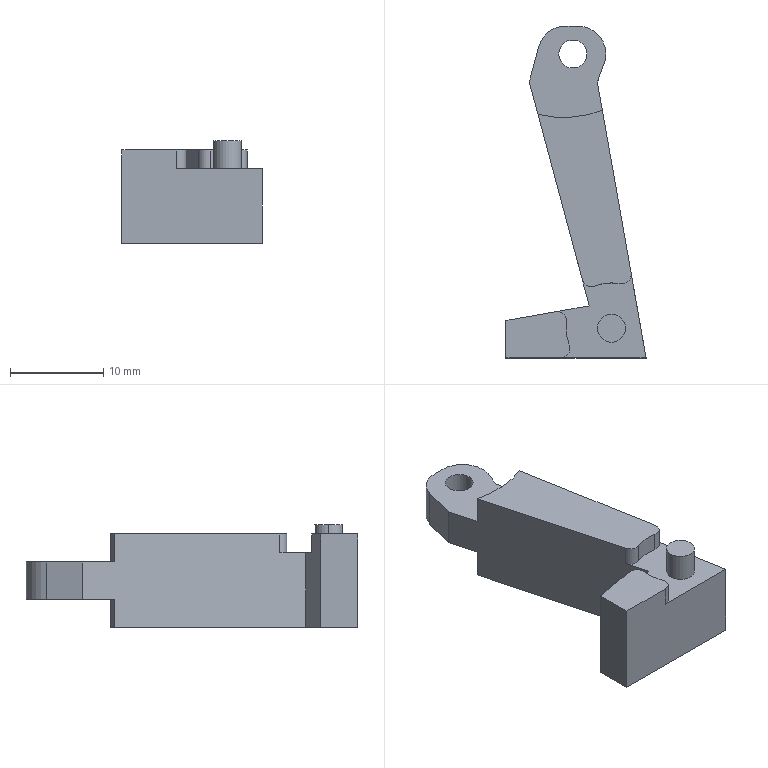Part | SolidWorks | features ICE 14, Fillet 5, MirrorPattern 2, Extrusion 1 | 1 solid | 33 faces | box 15 x 35.544 x 11 mm | volume 2110 mm3 | cylinder 18 | plane 15 | commonest cylinder face diameters 2 x7 3 x4 6 x3 9.731 x2 23.6 x2
STEP:
#1=CARTESIAN_POINT('',(13.411,8.923,8.));
#2=VERTEX_POINT('',#1);
#3=CARTESIAN_POINT('',(12.222,7.941,8.));
#4=VERTEX_POINT('',#3);
#5=CARTESIAN_POINT('',(12.411,8.923,8.));
#6=DIRECTION('',(0.,0.,-1.));
#7=DIRECTION('',(1.,0.,0.));
#8=AXIS2_PLACEMENT_3D('',#5,#6,#7);
#9=CIRCLE('',#8,1.);
#10=EDGE_CURVE('',#2,#4,#9,.T.);
#11=ORIENTED_EDGE('',*,*,#10,.F.);
#12=CARTESIAN_POINT('',(13.411,8.923,10.));
#13=VERTEX_POINT('',#12);
#14=CARTESIAN_POINT('',(13.411,8.923,8.));
#15=DIRECTION('',(0.,0.,1.));
#16=VECTOR('',#15,1000.);
#17=LINE('',#14,#16);
#18=EDGE_CURVE('',#2,#13,#17,.T.);
#19=ORIENTED_EDGE('',*,*,#18,.T.);
#20=CARTESIAN_POINT('',(12.222,7.941,10.));
#21=VERTEX_POINT('',#20);
#22=CARTESIAN_POINT('',(12.411,8.923,10.));
#23=DIRECTION('',(0.,0.,1.));
#24=DIRECTION('',(1.,0.,0.));
#25=AXIS2_PLACEMENT_3D('',#22,#23,#24);
#26=CIRCLE('',#25,1.);
#27=EDGE_CURVE('',#21,#13,#26,.T.);
#28=ORIENTED_EDGE('',*,*,#27,.F.);
#29=CARTESIAN_POINT('',(12.222,7.941,8.));
#30=DIRECTION('',(0.,0.,1.));
#31=VECTOR('',#30,1000.);
#32=LINE('',#29,#31);
#33=EDGE_CURVE('',#4,#21,#32,.T.);
#34=ORIENTED_EDGE('',*,*,#33,.F.);
#35=EDGE_LOOP('',(#11,#19,#28,#34));
#36=FACE_OUTER_BOUND('',#35,.T.);
#37=CARTESIAN_POINT('',(12.411,8.923,8.));
#38=DIRECTION('',(0.,0.,1.));
#39=DIRECTION('',(1.,0.,0.));
#40=AXIS2_PLACEMENT_3D('',#37,#38,#39);
#41=CYLINDRICAL_SURFACE('',#40,1.);
#42=ADVANCED_FACE('',(#36),#41,.T.);
#43=CARTESIAN_POINT('',(6.491,3.953,8.));
#44=VERTEX_POINT('',#43);
#45=CARTESIAN_POINT('',(6.482,3.818,8.));
#46=VERTEX_POINT('',#45);
#47=CARTESIAN_POINT('',(5.491,3.953,8.));
#48=DIRECTION('',(0.,0.,-1.));
#49=DIRECTION('',(1.,0.,0.));
#50=AXIS2_PLACEMENT_3D('',#47,#48,#49);
#51=CIRCLE('',#50,1.);
#52=EDGE_CURVE('',#44,#46,#51,.T.);
#53=ORIENTED_EDGE('',*,*,#52,.F.);
#54=CARTESIAN_POINT('',(6.491,3.953,10.));
#55=VERTEX_POINT('',#54);
#56=CARTESIAN_POINT('',(6.491,3.953,8.));
#57=DIRECTION('',(0.,0.,1.));
#58=VECTOR('',#57,1000.);
#59=LINE('',#56,#58);
#60=EDGE_CURVE('',#44,#55,#59,.T.);
#61=ORIENTED_EDGE('',*,*,#60,.T.);
#62=CARTESIAN_POINT('',(6.482,3.818,10.));
#63=VERTEX_POINT('',#62);
#64=CARTESIAN_POINT('',(5.491,3.953,10.));
#65=DIRECTION('',(0.,0.,1.));
#66=DIRECTION('',(1.,0.,0.));
#67=AXIS2_PLACEMENT_3D('',#64,#65,#66);
#68=CIRCLE('',#67,1.);
#69=EDGE_CURVE('',#63,#55,#68,.T.);
#70=ORIENTED_EDGE('',*,*,#69,.F.);
#71=CARTESIAN_POINT('',(6.482,3.818,8.));
#72=DIRECTION('',(0.,0.,1.));
#73=VECTOR('',#72,1000.);
#74=LINE('',#71,#73);
#75=EDGE_CURVE('',#46,#63,#74,.T.);
#76=ORIENTED_EDGE('',*,*,#75,.F.);
#77=EDGE_LOOP('',(#53,#61,#70,#76));
#78=FACE_OUTER_BOUND('',#77,.T.);
#79=CARTESIAN_POINT('',(5.491,3.953,8.));
#80=DIRECTION('',(0.,0.,1.));
#81=DIRECTION('',(1.,0.,0.));
#82=AXIS2_PLACEMENT_3D('',#79,#80,#81);
#83=CYLINDRICAL_SURFACE('',#82,1.);
#84=ADVANCED_FACE('',(#78),#83,.T.);
#85=CARTESIAN_POINT('',(6.851,1.,8.));
#86=VERTEX_POINT('',#85);
#87=CARTESIAN_POINT('',(5.851,0.,8.));
#88=VERTEX_POINT('',#87);
#89=CARTESIAN_POINT('',(5.851,1.,8.));
#90=DIRECTION('',(0.,0.,-1.));
#91=DIRECTION('',(1.,0.,0.));
#92=AXIS2_PLACEMENT_3D('',#89,#90,#91);
#93=CIRCLE('',#92,1.);
#94=EDGE_CURVE('',#86,#88,#93,.T.);
#95=ORIENTED_EDGE('',*,*,#94,.F.);
#96=CARTESIAN_POINT('',(6.851,1.,10.));
#97=VERTEX_POINT('',#96);
#98=CARTESIAN_POINT('',(6.851,1.,8.));
#99=DIRECTION('',(0.,0.,1.));
#100=VECTOR('',#99,1000.);
#101=LINE('',#98,#100);
#102=EDGE_CURVE('',#86,#97,#101,.T.);
#103=ORIENTED_EDGE('',*,*,#102,.T.);
#104=CARTESIAN_POINT('',(5.851,0.,10.));
#105=VERTEX_POINT('',#104);
#106=CARTESIAN_POINT('',(5.851,1.,10.));
#107=DIRECTION('',(0.,0.,1.));
#108=DIRECTION('',(1.,0.,0.));
#109=AXIS2_PLACEMENT_3D('',#106,#107,#108);
#110=CIRCLE('',#109,1.);
#111=EDGE_CURVE('',#105,#97,#110,.T.);
#112=ORIENTED_EDGE('',*,*,#111,.F.);
#113=CARTESIAN_POINT('',(5.851,0.,10.));
#114=DIRECTION('',(0.,0.,1.));
#115=VECTOR('',#114,1000.);
#116=LINE('',#113,#115);
#117=EDGE_CURVE('',#88,#105,#116,.T.);
#118=ORIENTED_EDGE('',*,*,#117,.F.);
#119=EDGE_LOOP('',(#95,#103,#112,#118));
#120=FACE_OUTER_BOUND('',#119,.T.);
#121=CARTESIAN_POINT('',(5.851,1.,8.));
#122=DIRECTION('',(0.,0.,1.));
#123=DIRECTION('',(1.,0.,0.));
#124=AXIS2_PLACEMENT_3D('',#121,#122,#123);
#125=CYLINDRICAL_SURFACE('',#124,1.);
#126=ADVANCED_FACE('',(#120),#125,.T.);
#127=CARTESIAN_POINT('',(12.803,3.163,11.));
#128=VERTEX_POINT('',#127);
#129=CARTESIAN_POINT('',(9.803,3.163,11.));
#130=VERTEX_POINT('',#129);
#131=CARTESIAN_POINT('',(11.303,3.163,11.));
#132=DIRECTION('',(0.,0.,1.));
#133=DIRECTION('',(1.,0.,0.));
#134=AXIS2_PLACEMENT_3D('',#131,#132,#133);
#135=CIRCLE('',#134,1.5);
#136=EDGE_CURVE('',#128,#130,#135,.T.);
#137=ORIENTED_EDGE('',*,*,#136,.F.);
#138=CARTESIAN_POINT('',(12.803,3.163,8.));
#139=VERTEX_POINT('',#138);
#140=CARTESIAN_POINT('',(12.803,3.163,11.));
#141=DIRECTION('',(0.,0.,-1.));
#142=VECTOR('',#141,1000.);
#143=LINE('',#140,#142);
#144=EDGE_CURVE('',#128,#139,#143,.T.);
#145=ORIENTED_EDGE('',*,*,#144,.T.);
#146=CARTESIAN_POINT('',(9.803,3.163,8.));
#147=VERTEX_POINT('',#146);
#148=CARTESIAN_POINT('',(11.303,3.163,8.));
#149=DIRECTION('',(0.,0.,1.));
#150=DIRECTION('',(1.,0.,0.));
#151=AXIS2_PLACEMENT_3D('',#148,#149,#150);
#152=CIRCLE('',#151,1.5);
#153=EDGE_CURVE('',#139,#147,#152,.T.);
#154=ORIENTED_EDGE('',*,*,#153,.T.);
#155=CARTESIAN_POINT('',(9.803,3.163,11.));
#156=DIRECTION('',(0.,0.,-1.));
#157=VECTOR('',#156,1000.);
#158=LINE('',#155,#157);
#159=EDGE_CURVE('',#130,#147,#158,.T.);
#160=ORIENTED_EDGE('',*,*,#159,.F.);
#161=EDGE_LOOP('',(#137,#145,#154,#160));
#162=FACE_OUTER_BOUND('',#161,.T.);
#163=CARTESIAN_POINT('',(11.303,3.163,11.));
#164=DIRECTION('',(0.,0.,-1.));
#165=DIRECTION('',(-1.,0.,0.));
#166=AXIS2_PLACEMENT_3D('',#163,#164,#165);
#167=CYLINDRICAL_SURFACE('',#166,1.5);
#168=ADVANCED_FACE('',(#162),#167,.T.);
#169=CARTESIAN_POINT('',(8.658,32.544,7.));
#170=VERTEX_POINT('',#169);
#171=CARTESIAN_POINT('',(5.658,32.544,7.));
#172=VERTEX_POINT('',#171);
#173=CARTESIAN_POINT('',(7.158,32.544,7.));
#174=DIRECTION('',(0.,0.,-1.));
#175=DIRECTION('',(0.,-1.,0.));
#176=AXIS2_PLACEMENT_3D('',#173,#174,#175);
#177=CIRCLE('',#176,1.5);
#178=EDGE_CURVE('',#170,#172,#177,.T.);
#179=ORIENTED_EDGE('',*,*,#178,.F.);
#180=CARTESIAN_POINT('',(8.658,32.544,3.));
#181=VERTEX_POINT('',#180);
#182=CARTESIAN_POINT('',(8.658,32.544,30.));
#183=DIRECTION('',(0.,0.,-1.));
#184=VECTOR('',#183,1000.);
#185=LINE('',#182,#184);
#186=EDGE_CURVE('',#170,#181,#185,.T.);
#187=ORIENTED_EDGE('',*,*,#186,.T.);
#188=CARTESIAN_POINT('',(5.658,32.544,3.));
#189=VERTEX_POINT('',#188);
#190=CARTESIAN_POINT('',(7.158,32.544,3.));
#191=DIRECTION('',(0.,0.,1.));
#192=DIRECTION('',(0.,1.,0.));
#193=AXIS2_PLACEMENT_3D('',#190,#191,#192);
#194=CIRCLE('',#193,1.5);
#195=EDGE_CURVE('',#189,#181,#194,.T.);
#196=ORIENTED_EDGE('',*,*,#195,.F.);
#197=CARTESIAN_POINT('',(5.658,32.544,30.));
#198=DIRECTION('',(0.,0.,-1.));
#199=VECTOR('',#198,1000.);
#200=LINE('',#197,#199);
#201=EDGE_CURVE('',#172,#189,#200,.T.);
#202=ORIENTED_EDGE('',*,*,#201,.F.);
#203=EDGE_LOOP('',(#179,#187,#196,#202));
#204=FACE_OUTER_BOUND('',#203,.T.);
#205=CARTESIAN_POINT('',(7.158,32.544,30.));
#206=DIRECTION('',(0.,0.,-1.));
#207=DIRECTION('',(-1.,0.,0.));
#208=AXIS2_PLACEMENT_3D('',#205,#206,#207);
#209=CYLINDRICAL_SURFACE('',#208,1.5);
#210=ADVANCED_FACE('',(#204),#209,.F.);
#211=CARTESIAN_POINT('',(10.509,31.518,3.));
#212=VERTEX_POINT('',#211);
#213=CARTESIAN_POINT('',(10.69,32.544,3.));
#214=VERTEX_POINT('',#213);
#215=CARTESIAN_POINT('',(7.69,32.544,3.));
#216=DIRECTION('',(0.,0.,1.));
#217=DIRECTION('',(0.,1.,0.));
#218=AXIS2_PLACEMENT_3D('',#215,#216,#217);
#219=CIRCLE('',#218,3.);
#220=EDGE_CURVE('',#212,#214,#219,.T.);
#221=ORIENTED_EDGE('',*,*,#220,.T.);
#222=CARTESIAN_POINT('',(10.69,32.544,7.));
#223=VERTEX_POINT('',#222);
#224=CARTESIAN_POINT('',(10.69,32.544,10.));
#225=DIRECTION('',(0.,0.,1.));
#226=VECTOR('',#225,1000.);
#227=LINE('',#224,#226);
#228=EDGE_CURVE('',#214,#223,#227,.T.);
#229=ORIENTED_EDGE('',*,*,#228,.T.);
#230=CARTESIAN_POINT('',(10.509,31.518,7.));
#231=VERTEX_POINT('',#230);
#232=CARTESIAN_POINT('',(7.69,32.544,7.));
#233=DIRECTION('',(0.,0.,-1.));
#234=DIRECTION('',(0.,-1.,0.));
#235=AXIS2_PLACEMENT_3D('',#232,#233,#234);
#236=CIRCLE('',#235,3.);
#237=EDGE_CURVE('',#223,#231,#236,.T.);
#238=ORIENTED_EDGE('',*,*,#237,.T.);
#239=CARTESIAN_POINT('',(10.509,31.518,10.));
#240=DIRECTION('',(0.,0.,1.));
#241=VECTOR('',#240,1000.);
#242=LINE('',#239,#241);
#243=EDGE_CURVE('',#212,#231,#242,.T.);
#244=ORIENTED_EDGE('',*,*,#243,.F.);
#245=EDGE_LOOP('',(#221,#229,#238,#244));
#246=FACE_OUTER_BOUND('',#245,.T.);
#247=CARTESIAN_POINT('',(7.69,32.544,10.));
#248=DIRECTION('',(0.,0.,1.));
#249=DIRECTION('',(1.,0.,0.));
#250=AXIS2_PLACEMENT_3D('',#247,#248,#249);
#251=CYLINDRICAL_SURFACE('',#250,3.);
#252=ADVANCED_FACE('',(#246),#251,.T.);
#253=CARTESIAN_POINT('',(3.431,26.06,10.));
#254=VERTEX_POINT('',#253);
#255=CARTESIAN_POINT('',(8.175,8.356,10.));
#256=VERTEX_POINT('',#255);
#257=CARTESIAN_POINT('',(2.497,29.544,10.));
#258=DIRECTION('',(0.2588,-0.9659,0.));
#259=VECTOR('',#258,1000.);
#260=LINE('',#257,#259);
#261=EDGE_CURVE('',#254,#256,#260,.T.);
#262=ORIENTED_EDGE('',*,*,#261,.T.);
#263=CARTESIAN_POINT('',(9.509,7.686,10.));
#264=VERTEX_POINT('',#263);
#265=CARTESIAN_POINT('',(9.141,8.615,10.));
#266=DIRECTION('',(0.,0.,1.));
#267=DIRECTION('',(1.,0.,0.));
#268=AXIS2_PLACEMENT_3D('',#265,#266,#267);
#269=CIRCLE('',#268,1.);
#270=EDGE_CURVE('',#256,#264,#269,.T.);
#271=ORIENTED_EDGE('',*,*,#270,.T.);
#272=CARTESIAN_POINT('',(11.303,3.163,10.));
#273=DIRECTION('',(0.,0.,1.));
#274=DIRECTION('',(1.,0.,0.));
#275=AXIS2_PLACEMENT_3D('',#272,#273,#274);
#276=CIRCLE('',#275,4.865);
#277=EDGE_CURVE('',#21,#264,#276,.T.);
#278=ORIENTED_EDGE('',*,*,#277,.F.);
#279=ORIENTED_EDGE('',*,*,#27,.T.);
#280=CARTESIAN_POINT('',(13.396,9.097,10.));
#281=VERTEX_POINT('',#280);
#282=CARTESIAN_POINT('',(12.411,8.923,10.));
#283=DIRECTION('',(0.,0.,1.));
#284=DIRECTION('',(1.,0.,0.));
#285=AXIS2_PLACEMENT_3D('',#282,#283,#284);
#286=CIRCLE('',#285,1.);
#287=EDGE_CURVE('',#13,#281,#286,.T.);
#288=ORIENTED_EDGE('',*,*,#287,.T.);
#289=CARTESIAN_POINT('',(10.326,26.51,10.));
#290=VERTEX_POINT('',#289);
#291=CARTESIAN_POINT('',(15.,0.,10.));
#292=DIRECTION('',(-0.1736,0.9848,0.));
#293=VECTOR('',#292,1000.);
#294=LINE('',#291,#293);
#295=EDGE_CURVE('',#281,#290,#294,.T.);
#296=ORIENTED_EDGE('',*,*,#295,.T.);
#297=CARTESIAN_POINT('',(6.144,37.544,10.));
#298=DIRECTION('',(0.,0.,-1.));
#299=DIRECTION('',(-1.,0.,0.));
#300=AXIS2_PLACEMENT_3D('',#297,#298,#299);
#301=CIRCLE('',#300,11.8);
#302=EDGE_CURVE('',#290,#254,#301,.T.);
#303=ORIENTED_EDGE('',*,*,#302,.T.);
#304=EDGE_LOOP('',(#262,#271,#278,#279,#288,#296,#303));
#305=FACE_OUTER_BOUND('',#304,.T.);
#306=CARTESIAN_POINT('',(0.,0.,10.));
#307=DIRECTION('',(0.,0.,1.));
#308=DIRECTION('',(1.,0.,0.));
#309=AXIS2_PLACEMENT_3D('',#306,#307,#308);
#310=PLANE('',#309);
#311=ADVANCED_FACE('',(#305),#310,.T.);
#312=CARTESIAN_POINT('',(0.,0.,10.));
#313=VERTEX_POINT('',#312);
#314=CARTESIAN_POINT('',(0.,0.,10.));
#315=DIRECTION('',(1.,0.,0.));
#316=VECTOR('',#315,1000.);
#317=LINE('',#314,#316);
#318=EDGE_CURVE('',#313,#105,#317,.T.);
#319=ORIENTED_EDGE('',*,*,#318,.T.);
#320=ORIENTED_EDGE('',*,*,#111,.T.);
#321=CARTESIAN_POINT('',(6.781,1.369,10.));
#322=VERTEX_POINT('',#321);
#323=CARTESIAN_POINT('',(5.851,1.,10.));
#324=DIRECTION('',(0.,0.,1.));
#325=DIRECTION('',(1.,0.,0.));
#326=AXIS2_PLACEMENT_3D('',#323,#324,#325);
#327=CIRCLE('',#326,1.);
#328=EDGE_CURVE('',#97,#322,#327,.T.);
#329=ORIENTED_EDGE('',*,*,#328,.T.);
#330=CARTESIAN_POINT('',(11.303,3.163,10.));
#331=DIRECTION('',(0.,0.,1.));
#332=DIRECTION('',(1.,0.,0.));
#333=AXIS2_PLACEMENT_3D('',#330,#331,#332);
#334=CIRCLE('',#333,4.865);
#335=EDGE_CURVE('',#63,#322,#334,.T.);
#336=ORIENTED_EDGE('',*,*,#335,.F.);
#337=ORIENTED_EDGE('',*,*,#69,.T.);
#338=CARTESIAN_POINT('',(5.318,4.938,10.));
#339=VERTEX_POINT('',#338);
#340=CARTESIAN_POINT('',(5.491,3.953,10.));
#341=DIRECTION('',(0.,0.,1.));
#342=DIRECTION('',(1.,0.,0.));
#343=AXIS2_PLACEMENT_3D('',#340,#341,#342);
#344=CIRCLE('',#343,1.);
#345=EDGE_CURVE('',#55,#339,#344,.T.);
#346=ORIENTED_EDGE('',*,*,#345,.T.);
#347=CARTESIAN_POINT('',(0.,4.,10.));
#348=VERTEX_POINT('',#347);
#349=CARTESIAN_POINT('',(8.921,5.573,10.));
#350=DIRECTION('',(-0.9848,-0.1736,0.));
#351=VECTOR('',#350,1000.);
#352=LINE('',#349,#351);
#353=EDGE_CURVE('',#339,#348,#352,.T.);
#354=ORIENTED_EDGE('',*,*,#353,.T.);
#355=CARTESIAN_POINT('',(0.,4.,10.));
#356=DIRECTION('',(0.,-1.,0.));
#357=VECTOR('',#356,1000.);
#358=LINE('',#355,#357);
#359=EDGE_CURVE('',#348,#313,#358,.T.);
#360=ORIENTED_EDGE('',*,*,#359,.T.);
#361=EDGE_LOOP('',(#319,#320,#329,#336,#337,#346,#354,#360));
#362=FACE_OUTER_BOUND('',#361,.T.);
#363=CARTESIAN_POINT('',(0.,0.,10.));
#364=DIRECTION('',(0.,0.,1.));
#365=DIRECTION('',(1.,0.,0.));
#366=AXIS2_PLACEMENT_3D('',#363,#364,#365);
#367=PLANE('',#366);
#368=ADVANCED_FACE('',(#362),#367,.T.);
#369=ORIENTED_EDGE('',*,*,#295,.F.);
#370=CARTESIAN_POINT('',(13.396,9.097,8.));
#371=VERTEX_POINT('',#370);
#372=CARTESIAN_POINT('',(13.396,9.097,10.));
#373=DIRECTION('',(0.,0.,-1.));
#374=VECTOR('',#373,1000.);
#375=LINE('',#372,#374);
#376=EDGE_CURVE('',#281,#371,#375,.T.);
#377=ORIENTED_EDGE('',*,*,#376,.T.);
#378=CARTESIAN_POINT('',(15.,0.,8.));
#379=VERTEX_POINT('',#378);
#380=CARTESIAN_POINT('',(15.,0.,8.));
#381=DIRECTION('',(-0.1736,0.9848,0.));
#382=VECTOR('',#381,1000.);
#383=LINE('',#380,#382);
#384=EDGE_CURVE('',#379,#371,#383,.T.);
#385=ORIENTED_EDGE('',*,*,#384,.F.);
#386=CARTESIAN_POINT('',(15.,0.,0.));
#387=VERTEX_POINT('',#386);
#388=CARTESIAN_POINT('',(15.,0.,10.));
#389=DIRECTION('',(0.,0.,-1.));
#390=VECTOR('',#389,1000.);
#391=LINE('',#388,#390);
#392=EDGE_CURVE('',#379,#387,#391,.T.);
#393=ORIENTED_EDGE('',*,*,#392,.T.);
#394=CARTESIAN_POINT('',(10.326,26.51,0.));
#395=VERTEX_POINT('',#394);
#396=CARTESIAN_POINT('',(15.,0.,0.));
#397=DIRECTION('',(-0.1736,0.9848,0.));
#398=VECTOR('',#397,1000.);
#399=LINE('',#396,#398);
#400=EDGE_CURVE('',#387,#395,#399,.T.);
#401=ORIENTED_EDGE('',*,*,#400,.T.);
#402=CARTESIAN_POINT('',(10.326,26.51,3.));
#403=VERTEX_POINT('',#402);
#404=CARTESIAN_POINT('',(10.326,26.51,3.));
#405=DIRECTION('',(0.,0.,-1.));
#406=VECTOR('',#405,1000.);
#407=LINE('',#404,#406);
#408=EDGE_CURVE('',#403,#395,#407,.T.);
#409=ORIENTED_EDGE('',*,*,#408,.F.);
#410=CARTESIAN_POINT('',(9.791,29.544,3.));
#411=VERTEX_POINT('',#410);
#412=CARTESIAN_POINT('',(14.548,2.565,3.));
#413=DIRECTION('',(0.1736,-0.9848,0.));
#414=VECTOR('',#413,1000.);
#415=LINE('',#412,#414);
#416=EDGE_CURVE('',#411,#403,#415,.T.);
#417=ORIENTED_EDGE('',*,*,#416,.F.);
#418=CARTESIAN_POINT('',(9.791,29.544,7.));
#419=VERTEX_POINT('',#418);
#420=CARTESIAN_POINT('',(9.791,29.544,10.));
#421=DIRECTION('',(0.,0.,-1.));
#422=VECTOR('',#421,1000.);
#423=LINE('',#420,#422);
#424=EDGE_CURVE('',#419,#411,#423,.T.);
#425=ORIENTED_EDGE('',*,*,#424,.F.);
#426=CARTESIAN_POINT('',(10.326,26.51,7.));
#427=VERTEX_POINT('',#426);
#428=CARTESIAN_POINT('',(14.548,2.565,7.));
#429=DIRECTION('',(0.1736,-0.9848,0.));
#430=VECTOR('',#429,1000.);
#431=LINE('',#428,#430);
#432=EDGE_CURVE('',#419,#427,#431,.T.);
#433=ORIENTED_EDGE('',*,*,#432,.T.);
#434=CARTESIAN_POINT('',(10.326,26.51,7.));
#435=DIRECTION('',(0.,0.,1.));
#436=VECTOR('',#435,1000.);
#437=LINE('',#434,#436);
#438=EDGE_CURVE('',#427,#290,#437,.T.);
#439=ORIENTED_EDGE('',*,*,#438,.T.);
#440=EDGE_LOOP('',(#369,#377,#385,#393,#401,#409,#417,#425,#433,#439));
#441=FACE_OUTER_BOUND('',#440,.T.);
#442=CARTESIAN_POINT('',(15.,0.,10.));
#443=DIRECTION('',(-0.9848,-0.1736,0.));
#444=DIRECTION('',(0.1736,-0.9848,0.));
#445=AXIS2_PLACEMENT_3D('',#442,#443,#444);
#446=PLANE('',#445);
#447=ADVANCED_FACE('',(#441),#446,.F.);
#448=CARTESIAN_POINT('',(8.175,8.356,8.));
#449=VERTEX_POINT('',#448);
#450=CARTESIAN_POINT('',(8.921,5.573,8.));
#451=VERTEX_POINT('',#450);
#452=CARTESIAN_POINT('',(2.497,29.544,8.));
#453=DIRECTION('',(0.2588,-0.9659,0.));
#454=VECTOR('',#453,1000.);
#455=LINE('',#452,#454);
#456=EDGE_CURVE('',#449,#451,#455,.T.);
#457=ORIENTED_EDGE('',*,*,#456,.F.);
#458=CARTESIAN_POINT('',(8.175,8.356,10.));
#459=DIRECTION('',(0.,0.,1.));
#460=VECTOR('',#459,1000.);
#461=LINE('',#458,#460);
#462=EDGE_CURVE('',#449,#256,#461,.T.);
#463=ORIENTED_EDGE('',*,*,#462,.T.);
#464=ORIENTED_EDGE('',*,*,#261,.F.);
#465=CARTESIAN_POINT('',(3.431,26.06,7.));
#466=VERTEX_POINT('',#465);
#467=CARTESIAN_POINT('',(3.431,26.06,7.));
#468=DIRECTION('',(0.,0.,1.));
#469=VECTOR('',#468,1000.);
#470=LINE('',#467,#469);
#471=EDGE_CURVE('',#466,#254,#470,.T.);
#472=ORIENTED_EDGE('',*,*,#471,.F.);
#473=CARTESIAN_POINT('',(2.497,29.544,7.));
#474=VERTEX_POINT('',#473);
#475=CARTESIAN_POINT('',(9.716,2.603,7.));
#476=DIRECTION('',(-0.2588,0.9659,0.));
#477=VECTOR('',#476,1000.);
#478=LINE('',#475,#477);
#479=EDGE_CURVE('',#466,#474,#478,.T.);
#480=ORIENTED_EDGE('',*,*,#479,.T.);
#481=CARTESIAN_POINT('',(2.497,29.544,3.));
#482=VERTEX_POINT('',#481);
#483=CARTESIAN_POINT('',(2.497,29.544,10.));
#484=DIRECTION('',(0.,0.,-1.));
#485=VECTOR('',#484,1000.);
#486=LINE('',#483,#485);
#487=EDGE_CURVE('',#474,#482,#486,.T.);
#488=ORIENTED_EDGE('',*,*,#487,.T.);
#489=CARTESIAN_POINT('',(3.431,26.06,3.));
#490=VERTEX_POINT('',#489);
#491=CARTESIAN_POINT('',(9.716,2.603,3.));
#492=DIRECTION('',(-0.2588,0.9659,0.));
#493=VECTOR('',#492,1000.);
#494=LINE('',#491,#493);
#495=EDGE_CURVE('',#490,#482,#494,.T.);
#496=ORIENTED_EDGE('',*,*,#495,.F.);
#497=CARTESIAN_POINT('',(3.431,26.06,0.));
#498=VERTEX_POINT('',#497);
#499=CARTESIAN_POINT('',(3.431,26.06,3.));
#500=DIRECTION('',(0.,0.,-1.));
#501=VECTOR('',#500,1000.);
#502=LINE('',#499,#501);
#503=EDGE_CURVE('',#490,#498,#502,.T.);
#504=ORIENTED_EDGE('',*,*,#503,.T.);
#505=CARTESIAN_POINT('',(8.921,5.573,0.));
#506=VERTEX_POINT('',#505);
#507=CARTESIAN_POINT('',(2.497,29.544,0.));
#508=DIRECTION('',(0.2588,-0.9659,0.));
#509=VECTOR('',#508,1000.);
#510=LINE('',#507,#509);
#511=EDGE_CURVE('',#498,#506,#510,.T.);
#512=ORIENTED_EDGE('',*,*,#511,.T.);
#513=CARTESIAN_POINT('',(8.921,5.573,10.));
#514=DIRECTION('',(0.,0.,-1.));
#515=VECTOR('',#514,1000.);
#516=LINE('',#513,#515);
#517=EDGE_CURVE('',#451,#506,#516,.T.);
#518=ORIENTED_EDGE('',*,*,#517,.F.);
#519=EDGE_LOOP('',(#457,#463,#464,#472,#480,#488,#496,#504,#512,#518));
#520=FACE_OUTER_BOUND('',#519,.T.);
#521=CARTESIAN_POINT('',(2.497,29.544,10.));
#522=DIRECTION('',(0.9659,0.2588,0.));
#523=DIRECTION('',(-0.2588,0.9659,0.));
#524=AXIS2_PLACEMENT_3D('',#521,#522,#523);
#525=PLANE('',#524);
#526=ADVANCED_FACE('',(#520),#525,.F.);
#527=CARTESIAN_POINT('',(9.791,29.544,7.));
#528=DIRECTION('',(0.342,0.9397,0.));
#529=VECTOR('',#528,1000.);
#530=LINE('',#527,#529);
#531=EDGE_CURVE('',#419,#231,#530,.T.);
#532=ORIENTED_EDGE('',*,*,#531,.F.);
#533=ORIENTED_EDGE('',*,*,#424,.T.);
#534=CARTESIAN_POINT('',(9.791,29.544,3.));
#535=DIRECTION('',(-0.342,-0.9397,0.));
#536=VECTOR('',#535,1000.);
#537=LINE('',#534,#536);
#538=EDGE_CURVE('',#212,#411,#537,.T.);
#539=ORIENTED_EDGE('',*,*,#538,.F.);
#540=ORIENTED_EDGE('',*,*,#243,.T.);
#541=EDGE_LOOP('',(#532,#533,#539,#540));
#542=FACE_OUTER_BOUND('',#541,.T.);
#543=CARTESIAN_POINT('',(9.791,29.544,10.));
#544=DIRECTION('',(-0.9397,0.342,0.));
#545=DIRECTION('',(-0.342,-0.9397,0.));
#546=AXIS2_PLACEMENT_3D('',#543,#544,#545);
#547=PLANE('',#546);
#548=ADVANCED_FACE('',(#542),#547,.F.);
#549=CARTESIAN_POINT('',(3.509,33.321,7.));
#550=VERTEX_POINT('',#549);
#551=CARTESIAN_POINT('',(10.051,57.735,7.));
#552=DIRECTION('',(-0.2588,-0.9659,0.));
#553=VECTOR('',#552,1000.);
#554=LINE('',#551,#553);
#555=EDGE_CURVE('',#550,#474,#554,.T.);
#556=ORIENTED_EDGE('',*,*,#555,.F.);
#557=CARTESIAN_POINT('',(3.509,33.321,3.));
#558=VERTEX_POINT('',#557);
#559=CARTESIAN_POINT('',(3.509,33.321,10.));
#560=DIRECTION('',(0.,0.,-1.));
#561=VECTOR('',#560,1000.);
#562=LINE('',#559,#561);
#563=EDGE_CURVE('',#550,#558,#562,.T.);
#564=ORIENTED_EDGE('',*,*,#563,.T.);
#565=CARTESIAN_POINT('',(10.051,57.735,3.));
#566=DIRECTION('',(0.2588,0.9659,0.));
#567=VECTOR('',#566,1000.);
#568=LINE('',#565,#567);
#569=EDGE_CURVE('',#482,#558,#568,.T.);
#570=ORIENTED_EDGE('',*,*,#569,.F.);
#571=ORIENTED_EDGE('',*,*,#487,.F.);
#572=EDGE_LOOP('',(#556,#564,#570,#571));
#573=FACE_OUTER_BOUND('',#572,.T.);
#574=CARTESIAN_POINT('',(10.051,57.735,10.));
#575=DIRECTION('',(0.9659,-0.2588,0.));
#576=DIRECTION('',(0.2588,0.9659,0.));
#577=AXIS2_PLACEMENT_3D('',#574,#575,#576);
#578=PLANE('',#577);
#579=ADVANCED_FACE('',(#573),#578,.F.);
#580=ORIENTED_EDGE('',*,*,#511,.F.);
#581=CARTESIAN_POINT('',(6.144,37.544,0.));
#582=DIRECTION('',(0.,0.,-1.));
#583=DIRECTION('',(-1.,0.,0.));
#584=AXIS2_PLACEMENT_3D('',#581,#582,#583);
#585=CIRCLE('',#584,11.8);
#586=EDGE_CURVE('',#395,#498,#585,.T.);
#587=ORIENTED_EDGE('',*,*,#586,.F.);
#588=ORIENTED_EDGE('',*,*,#400,.F.);
#589=CARTESIAN_POINT('',(0.,0.,0.));
#590=VERTEX_POINT('',#589);
#591=CARTESIAN_POINT('',(0.,0.,0.));
#592=DIRECTION('',(1.,0.,0.));
#593=VECTOR('',#592,1000.);
#594=LINE('',#591,#593);
#595=EDGE_CURVE('',#590,#387,#594,.T.);
#596=ORIENTED_EDGE('',*,*,#595,.F.);
#597=CARTESIAN_POINT('',(0.,4.,0.));
#598=VERTEX_POINT('',#597);
#599=CARTESIAN_POINT('',(0.,4.,0.));
#600=DIRECTION('',(0.,-1.,0.));
#601=VECTOR('',#600,1000.);
#602=LINE('',#599,#601);
#603=EDGE_CURVE('',#598,#590,#602,.T.);
#604=ORIENTED_EDGE('',*,*,#603,.F.);
#605=CARTESIAN_POINT('',(8.921,5.573,0.));
#606=DIRECTION('',(-0.9848,-0.1736,0.));
#607=VECTOR('',#606,1000.);
#608=LINE('',#605,#607);
#609=EDGE_CURVE('',#506,#598,#608,.T.);
#610=ORIENTED_EDGE('',*,*,#609,.F.);
#611=EDGE_LOOP('',(#580,#587,#588,#596,#604,#610));
#612=FACE_OUTER_BOUND('',#611,.T.);
#613=CARTESIAN_POINT('',(0.,0.,0.));
#614=DIRECTION('',(0.,0.,1.));
#615=DIRECTION('',(1.,0.,0.));
#616=AXIS2_PLACEMENT_3D('',#613,#614,#615);
#617=PLANE('',#616);
#618=ADVANCED_FACE('',(#612),#617,.F.);
#619=CARTESIAN_POINT('',(7.69,35.544,7.));
#620=VERTEX_POINT('',#619);
#621=CARTESIAN_POINT('',(6.407,35.544,7.));
#622=VERTEX_POINT('',#621);
#623=CARTESIAN_POINT('',(20.,35.544,7.));
#624=DIRECTION('',(-1.,0.,0.));
#625=VECTOR('',#624,1000.);
#626=LINE('',#623,#625);
#627=EDGE_CURVE('',#620,#622,#626,.T.);
#628=ORIENTED_EDGE('',*,*,#627,.F.);
#629=CARTESIAN_POINT('',(7.69,35.544,3.));
#630=VERTEX_POINT('',#629);
#631=CARTESIAN_POINT('',(7.69,35.544,30.));
#632=DIRECTION('',(0.,0.,-1.));
#633=VECTOR('',#632,1000.);
#634=LINE('',#631,#633);
#635=EDGE_CURVE('',#620,#630,#634,.T.);
#636=ORIENTED_EDGE('',*,*,#635,.T.);
#637=CARTESIAN_POINT('',(6.407,35.544,3.));
#638=VERTEX_POINT('',#637);
#639=CARTESIAN_POINT('',(20.,35.544,3.));
#640=DIRECTION('',(-1.,0.,0.));
#641=VECTOR('',#640,1000.);
#642=LINE('',#639,#641);
#643=EDGE_CURVE('',#630,#638,#642,.T.);
#644=ORIENTED_EDGE('',*,*,#643,.T.);
#645=CARTESIAN_POINT('',(6.407,35.544,30.));
#646=DIRECTION('',(0.,0.,1.));
#647=VECTOR('',#646,1000.);
#648=LINE('',#645,#647);
#649=EDGE_CURVE('',#638,#622,#648,.T.);
#650=ORIENTED_EDGE('',*,*,#649,.T.);
#651=EDGE_LOOP('',(#628,#636,#644,#650));
#652=FACE_OUTER_BOUND('',#651,.T.);
#653=CARTESIAN_POINT('',(4.105,35.544,30.));
#654=DIRECTION('',(0.,-1.,0.));
#655=DIRECTION('',(1.,0.,0.));
#656=AXIS2_PLACEMENT_3D('',#653,#654,#655);
#657=PLANE('',#656);
#658=ADVANCED_FACE('',(#652),#657,.F.);
#659=ORIENTED_EDGE('',*,*,#228,.F.);
#660=CARTESIAN_POINT('',(7.69,32.544,3.));
#661=DIRECTION('',(0.,0.,1.));
#662=DIRECTION('',(0.,1.,0.));
#663=AXIS2_PLACEMENT_3D('',#660,#661,#662);
#664=CIRCLE('',#663,3.);
#665=EDGE_CURVE('',#214,#630,#664,.T.);
#666=ORIENTED_EDGE('',*,*,#665,.T.);
#667=ORIENTED_EDGE('',*,*,#635,.F.);
#668=CARTESIAN_POINT('',(7.69,32.544,7.));
#669=DIRECTION('',(0.,0.,-1.));
#670=DIRECTION('',(0.,-1.,0.));
#671=AXIS2_PLACEMENT_3D('',#668,#669,#670);
#672=CIRCLE('',#671,3.);
#673=EDGE_CURVE('',#620,#223,#672,.T.);
#674=ORIENTED_EDGE('',*,*,#673,.T.);
#675=EDGE_LOOP('',(#659,#666,#667,#674));
#676=FACE_OUTER_BOUND('',#675,.T.);
#677=CARTESIAN_POINT('',(7.69,32.544,10.));
#678=DIRECTION('',(0.,0.,1.));
#679=DIRECTION('',(1.,0.,0.));
#680=AXIS2_PLACEMENT_3D('',#677,#678,#679);
#681=CYLINDRICAL_SURFACE('',#680,3.);
#682=ADVANCED_FACE('',(#676),#681,.T.);
#683=ORIENTED_EDGE('',*,*,#563,.F.);
#684=CARTESIAN_POINT('',(6.407,32.544,7.));
#685=DIRECTION('',(0.,0.,-1.));
#686=DIRECTION('',(0.,-1.,0.));
#687=AXIS2_PLACEMENT_3D('',#684,#685,#686);
#688=CIRCLE('',#687,3.);
#689=EDGE_CURVE('',#550,#622,#688,.T.);
#690=ORIENTED_EDGE('',*,*,#689,.T.);
#691=ORIENTED_EDGE('',*,*,#649,.F.);
#692=CARTESIAN_POINT('',(6.407,32.544,3.));
#693=DIRECTION('',(0.,0.,1.));
#694=DIRECTION('',(0.,1.,0.));
#695=AXIS2_PLACEMENT_3D('',#692,#693,#694);
#696=CIRCLE('',#695,3.);
#697=EDGE_CURVE('',#638,#558,#696,.T.);
#698=ORIENTED_EDGE('',*,*,#697,.T.);
#699=EDGE_LOOP('',(#683,#690,#691,#698));
#700=FACE_OUTER_BOUND('',#699,.T.);
#701=CARTESIAN_POINT('',(6.407,32.544,10.));
#702=DIRECTION('',(0.,0.,-1.));
#703=DIRECTION('',(-1.,0.,0.));
#704=AXIS2_PLACEMENT_3D('',#701,#702,#703);
#705=CYLINDRICAL_SURFACE('',#704,3.);
#706=ADVANCED_FACE('',(#700),#705,.T.);
#707=ORIENTED_EDGE('',*,*,#603,.T.);
#708=CARTESIAN_POINT('',(0.,0.,10.));
#709=DIRECTION('',(0.,0.,-1.));
#710=VECTOR('',#709,1000.);
#711=LINE('',#708,#710);
#712=EDGE_CURVE('',#313,#590,#711,.T.);
#713=ORIENTED_EDGE('',*,*,#712,.F.);
#714=ORIENTED_EDGE('',*,*,#359,.F.);
#715=CARTESIAN_POINT('',(0.,4.,10.));
#716=DIRECTION('',(0.,0.,-1.));
#717=VECTOR('',#716,1000.);
#718=LINE('',#715,#717);
#719=EDGE_CURVE('',#348,#598,#718,.T.);
#720=ORIENTED_EDGE('',*,*,#719,.T.);
#721=EDGE_LOOP('',(#707,#713,#714,#720));
#722=FACE_OUTER_BOUND('',#721,.T.);
#723=CARTESIAN_POINT('',(0.,4.,10.));
#724=DIRECTION('',(1.,0.,0.));
#725=DIRECTION('',(0.,1.,0.));
#726=AXIS2_PLACEMENT_3D('',#723,#724,#725);
#727=PLANE('',#726);
#728=ADVANCED_FACE('',(#722),#727,.F.);
#729=CARTESIAN_POINT('',(0.,0.,8.));
#730=DIRECTION('',(1.,0.,0.));
#731=VECTOR('',#730,1000.);
#732=LINE('',#729,#731);
#733=EDGE_CURVE('',#88,#379,#732,.T.);
#734=ORIENTED_EDGE('',*,*,#733,.F.);
#735=ORIENTED_EDGE('',*,*,#117,.T.);
#736=ORIENTED_EDGE('',*,*,#318,.F.);
#737=ORIENTED_EDGE('',*,*,#712,.T.);
#738=ORIENTED_EDGE('',*,*,#595,.T.);
#739=ORIENTED_EDGE('',*,*,#392,.F.);
#740=EDGE_LOOP('',(#734,#735,#736,#737,#738,#739));
#741=FACE_OUTER_BOUND('',#740,.T.);
#742=CARTESIAN_POINT('',(0.,0.,10.));
#743=DIRECTION('',(0.,1.,0.));
#744=DIRECTION('',(0.,0.,1.));
#745=AXIS2_PLACEMENT_3D('',#742,#743,#744);
#746=PLANE('',#745);
#747=ADVANCED_FACE('',(#741),#746,.F.);
#748=ORIENTED_EDGE('',*,*,#353,.F.);
#749=CARTESIAN_POINT('',(5.318,4.938,8.));
#750=VERTEX_POINT('',#749);
#751=CARTESIAN_POINT('',(5.318,4.938,10.));
#752=DIRECTION('',(0.,0.,-1.));
#753=VECTOR('',#752,1000.);
#754=LINE('',#751,#753);
#755=EDGE_CURVE('',#339,#750,#754,.T.);
#756=ORIENTED_EDGE('',*,*,#755,.T.);
#757=CARTESIAN_POINT('',(8.921,5.573,8.));
#758=DIRECTION('',(-0.9848,-0.1736,0.));
#759=VECTOR('',#758,1000.);
#760=LINE('',#757,#759);
#761=EDGE_CURVE('',#451,#750,#760,.T.);
#762=ORIENTED_EDGE('',*,*,#761,.F.);
#763=ORIENTED_EDGE('',*,*,#517,.T.);
#764=ORIENTED_EDGE('',*,*,#609,.T.);
#765=ORIENTED_EDGE('',*,*,#719,.F.);
#766=EDGE_LOOP('',(#748,#756,#762,#763,#764,#765));
#767=FACE_OUTER_BOUND('',#766,.T.);
#768=CARTESIAN_POINT('',(8.921,5.573,10.));
#769=DIRECTION('',(0.1736,-0.9848,0.));
#770=DIRECTION('',(0.9848,0.1736,0.));
#771=AXIS2_PLACEMENT_3D('',#768,#769,#770);
#772=PLANE('',#771);
#773=ADVANCED_FACE('',(#767),#772,.F.);
#774=ORIENTED_EDGE('',*,*,#538,.T.);
#775=ORIENTED_EDGE('',*,*,#416,.T.);
#776=CARTESIAN_POINT('',(6.144,37.544,3.));
#777=DIRECTION('',(0.,0.,-1.));
#778=DIRECTION('',(-1.,0.,0.));
#779=AXIS2_PLACEMENT_3D('',#776,#777,#778);
#780=CIRCLE('',#779,11.8);
#781=EDGE_CURVE('',#403,#490,#780,.T.);
#782=ORIENTED_EDGE('',*,*,#781,.T.);
#783=ORIENTED_EDGE('',*,*,#495,.T.);
#784=ORIENTED_EDGE('',*,*,#569,.T.);
#785=ORIENTED_EDGE('',*,*,#697,.F.);
#786=ORIENTED_EDGE('',*,*,#643,.F.);
#787=ORIENTED_EDGE('',*,*,#665,.F.);
#788=ORIENTED_EDGE('',*,*,#220,.F.);
#789=EDGE_LOOP('',(#774,#775,#782,#783,#784,#785,#786,#787,#788));
#790=FACE_OUTER_BOUND('',#789,.T.);
#791=ORIENTED_EDGE('',*,*,#195,.T.);
#792=CARTESIAN_POINT('',(7.158,32.544,3.));
#793=DIRECTION('',(0.,0.,1.));
#794=DIRECTION('',(0.,1.,0.));
#795=AXIS2_PLACEMENT_3D('',#792,#793,#794);
#796=CIRCLE('',#795,1.5);
#797=EDGE_CURVE('',#181,#189,#796,.T.);
#798=ORIENTED_EDGE('',*,*,#797,.T.);
#799=EDGE_LOOP('',(#791,#798));
#800=FACE_BOUND('',#799,.T.);
#801=CARTESIAN_POINT('',(20.,35.544,3.));
#802=DIRECTION('',(0.,0.,-1.));
#803=DIRECTION('',(0.,1.,0.));
#804=AXIS2_PLACEMENT_3D('',#801,#802,#803);
#805=PLANE('',#804);
#806=ADVANCED_FACE('',(#790,#800),#805,.T.);
#807=ORIENTED_EDGE('',*,*,#531,.T.);
#808=ORIENTED_EDGE('',*,*,#237,.F.);
#809=ORIENTED_EDGE('',*,*,#673,.F.);
#810=ORIENTED_EDGE('',*,*,#627,.T.);
#811=ORIENTED_EDGE('',*,*,#689,.F.);
#812=ORIENTED_EDGE('',*,*,#555,.T.);
#813=ORIENTED_EDGE('',*,*,#479,.F.);
#814=CARTESIAN_POINT('',(6.144,37.544,7.));
#815=DIRECTION('',(0.,0.,-1.));
#816=DIRECTION('',(-1.,0.,0.));
#817=AXIS2_PLACEMENT_3D('',#814,#815,#816);
#818=CIRCLE('',#817,11.8);
#819=EDGE_CURVE('',#427,#466,#818,.T.);
#820=ORIENTED_EDGE('',*,*,#819,.F.);
#821=ORIENTED_EDGE('',*,*,#432,.F.);
#822=EDGE_LOOP('',(#807,#808,#809,#810,#811,#812,#813,#820,#821));
#823=FACE_OUTER_BOUND('',#822,.T.);
#824=CARTESIAN_POINT('',(7.158,32.544,7.));
#825=DIRECTION('',(0.,0.,-1.));
#826=DIRECTION('',(0.,-1.,0.));
#827=AXIS2_PLACEMENT_3D('',#824,#825,#826);
#828=CIRCLE('',#827,1.5);
#829=EDGE_CURVE('',#172,#170,#828,.T.);
#830=ORIENTED_EDGE('',*,*,#829,.T.);
#831=ORIENTED_EDGE('',*,*,#178,.T.);
#832=EDGE_LOOP('',(#830,#831));
#833=FACE_BOUND('',#832,.T.);
#834=CARTESIAN_POINT('',(20.,35.544,7.));
#835=DIRECTION('',(0.,0.,1.));
#836=DIRECTION('',(0.,-1.,0.));
#837=AXIS2_PLACEMENT_3D('',#834,#835,#836);
#838=PLANE('',#837);
#839=ADVANCED_FACE('',(#823,#833),#838,.T.);
#840=ORIENTED_EDGE('',*,*,#186,.F.);
#841=ORIENTED_EDGE('',*,*,#829,.F.);
#842=ORIENTED_EDGE('',*,*,#201,.T.);
#843=ORIENTED_EDGE('',*,*,#797,.F.);
#844=EDGE_LOOP('',(#840,#841,#842,#843));
#845=FACE_OUTER_BOUND('',#844,.T.);
#846=CARTESIAN_POINT('',(7.158,32.544,30.));
#847=DIRECTION('',(0.,0.,-1.));
#848=DIRECTION('',(-1.,0.,0.));
#849=AXIS2_PLACEMENT_3D('',#846,#847,#848);
#850=CYLINDRICAL_SURFACE('',#849,1.5);
#851=ADVANCED_FACE('',(#845),#850,.F.);
#852=ORIENTED_EDGE('',*,*,#586,.T.);
#853=ORIENTED_EDGE('',*,*,#503,.F.);
#854=ORIENTED_EDGE('',*,*,#781,.F.);
#855=ORIENTED_EDGE('',*,*,#408,.T.);
#856=EDGE_LOOP('',(#852,#853,#854,#855));
#857=FACE_OUTER_BOUND('',#856,.T.);
#858=CARTESIAN_POINT('',(6.144,37.544,3.));
#859=DIRECTION('',(0.,0.,-1.));
#860=DIRECTION('',(-1.,0.,0.));
#861=AXIS2_PLACEMENT_3D('',#858,#859,#860);
#862=CYLINDRICAL_SURFACE('',#861,11.8);
#863=ADVANCED_FACE('',(#857),#862,.F.);
#864=ORIENTED_EDGE('',*,*,#302,.F.);
#865=ORIENTED_EDGE('',*,*,#438,.F.);
#866=ORIENTED_EDGE('',*,*,#819,.T.);
#867=ORIENTED_EDGE('',*,*,#471,.T.);
#868=EDGE_LOOP('',(#864,#865,#866,#867));
#869=FACE_OUTER_BOUND('',#868,.T.);
#870=CARTESIAN_POINT('',(6.144,37.544,7.));
#871=DIRECTION('',(0.,0.,1.));
#872=DIRECTION('',(1.,0.,0.));
#873=AXIS2_PLACEMENT_3D('',#870,#871,#872);
#874=CYLINDRICAL_SURFACE('',#873,11.8);
#875=ADVANCED_FACE('',(#869),#874,.F.);
#876=ORIENTED_EDGE('',*,*,#277,.T.);
#877=CARTESIAN_POINT('',(9.509,7.686,8.));
#878=VERTEX_POINT('',#877);
#879=CARTESIAN_POINT('',(9.509,7.686,8.));
#880=DIRECTION('',(0.,0.,-1.));
#881=VECTOR('',#880,1000.);
#882=LINE('',#879,#881);
#883=EDGE_CURVE('',#264,#878,#882,.T.);
#884=ORIENTED_EDGE('',*,*,#883,.T.);
#885=CARTESIAN_POINT('',(11.303,3.163,8.));
#886=DIRECTION('',(0.,0.,1.));
#887=DIRECTION('',(1.,0.,0.));
#888=AXIS2_PLACEMENT_3D('',#885,#886,#887);
#889=CIRCLE('',#888,4.865);
#890=EDGE_CURVE('',#4,#878,#889,.T.);
#891=ORIENTED_EDGE('',*,*,#890,.F.);
#892=ORIENTED_EDGE('',*,*,#33,.T.);
#893=EDGE_LOOP('',(#876,#884,#891,#892));
#894=FACE_OUTER_BOUND('',#893,.T.);
#895=CARTESIAN_POINT('',(11.303,3.163,8.));
#896=DIRECTION('',(0.,0.,1.));
#897=DIRECTION('',(1.,0.,0.));
#898=AXIS2_PLACEMENT_3D('',#895,#896,#897);
#899=CYLINDRICAL_SURFACE('',#898,4.865);
#900=ADVANCED_FACE('',(#894),#899,.F.);
#901=ORIENTED_EDGE('',*,*,#335,.T.);
#902=CARTESIAN_POINT('',(6.781,1.369,8.));
#903=VERTEX_POINT('',#902);
#904=CARTESIAN_POINT('',(6.781,1.369,8.));
#905=DIRECTION('',(0.,0.,-1.));
#906=VECTOR('',#905,1000.);
#907=LINE('',#904,#906);
#908=EDGE_CURVE('',#322,#903,#907,.T.);
#909=ORIENTED_EDGE('',*,*,#908,.T.);
#910=CARTESIAN_POINT('',(11.303,3.163,8.));
#911=DIRECTION('',(0.,0.,1.));
#912=DIRECTION('',(1.,0.,0.));
#913=AXIS2_PLACEMENT_3D('',#910,#911,#912);
#914=CIRCLE('',#913,4.865);
#915=EDGE_CURVE('',#46,#903,#914,.T.);
#916=ORIENTED_EDGE('',*,*,#915,.F.);
#917=ORIENTED_EDGE('',*,*,#75,.T.);
#918=EDGE_LOOP('',(#901,#909,#916,#917));
#919=FACE_OUTER_BOUND('',#918,.T.);
#920=CARTESIAN_POINT('',(11.303,3.163,8.));
#921=DIRECTION('',(0.,0.,1.));
#922=DIRECTION('',(1.,0.,0.));
#923=AXIS2_PLACEMENT_3D('',#920,#921,#922);
#924=CYLINDRICAL_SURFACE('',#923,4.865);
#925=ADVANCED_FACE('',(#919),#924,.F.);
#926=CARTESIAN_POINT('',(11.303,3.163,8.));
#927=DIRECTION('',(0.,0.,1.));
#928=DIRECTION('',(1.,0.,0.));
#929=AXIS2_PLACEMENT_3D('',#926,#927,#928);
#930=CIRCLE('',#929,1.5);
#931=EDGE_CURVE('',#147,#139,#930,.T.);
#932=ORIENTED_EDGE('',*,*,#931,.F.);
#933=ORIENTED_EDGE('',*,*,#153,.F.);
#934=EDGE_LOOP('',(#932,#933));
#935=FACE_BOUND('',#934,.T.);
#936=ORIENTED_EDGE('',*,*,#384,.T.);
#937=CARTESIAN_POINT('',(12.411,8.923,8.));
#938=DIRECTION('',(0.,0.,-1.));
#939=DIRECTION('',(1.,0.,0.));
#940=AXIS2_PLACEMENT_3D('',#937,#938,#939);
#941=CIRCLE('',#940,1.);
#942=EDGE_CURVE('',#371,#2,#941,.T.);
#943=ORIENTED_EDGE('',*,*,#942,.T.);
#944=ORIENTED_EDGE('',*,*,#10,.T.);
#945=ORIENTED_EDGE('',*,*,#890,.T.);
#946=CARTESIAN_POINT('',(9.141,8.615,8.));
#947=DIRECTION('',(0.,0.,-1.));
#948=DIRECTION('',(1.,0.,0.));
#949=AXIS2_PLACEMENT_3D('',#946,#947,#948);
#950=CIRCLE('',#949,1.);
#951=EDGE_CURVE('',#878,#449,#950,.T.);
#952=ORIENTED_EDGE('',*,*,#951,.T.);
#953=ORIENTED_EDGE('',*,*,#456,.T.);
#954=ORIENTED_EDGE('',*,*,#761,.T.);
#955=CARTESIAN_POINT('',(5.491,3.953,8.));
#956=DIRECTION('',(0.,0.,-1.));
#957=DIRECTION('',(1.,0.,0.));
#958=AXIS2_PLACEMENT_3D('',#955,#956,#957);
#959=CIRCLE('',#958,1.);
#960=EDGE_CURVE('',#750,#44,#959,.T.);
#961=ORIENTED_EDGE('',*,*,#960,.T.);
#962=ORIENTED_EDGE('',*,*,#52,.T.);
#963=ORIENTED_EDGE('',*,*,#915,.T.);
#964=CARTESIAN_POINT('',(5.851,1.,8.));
#965=DIRECTION('',(0.,0.,-1.));
#966=DIRECTION('',(1.,0.,0.));
#967=AXIS2_PLACEMENT_3D('',#964,#965,#966);
#968=CIRCLE('',#967,1.);
#969=EDGE_CURVE('',#903,#86,#968,.T.);
#970=ORIENTED_EDGE('',*,*,#969,.T.);
#971=ORIENTED_EDGE('',*,*,#94,.T.);
#972=ORIENTED_EDGE('',*,*,#733,.T.);
#973=EDGE_LOOP('',(#936,#943,#944,#945,#952,#953,#954,#961,#962,#963,#970,#971,#972));
#974=FACE_OUTER_BOUND('',#973,.T.);
#975=CARTESIAN_POINT('',(11.303,3.163,8.));
#976=DIRECTION('',(0.,0.,1.));
#977=DIRECTION('',(1.,0.,0.));
#978=AXIS2_PLACEMENT_3D('',#975,#976,#977);
#979=PLANE('',#978);
#980=ADVANCED_FACE('',(#935,#974),#979,.T.);
#981=CARTESIAN_POINT('',(11.303,3.163,11.));
#982=DIRECTION('',(0.,0.,1.));
#983=DIRECTION('',(1.,0.,0.));
#984=AXIS2_PLACEMENT_3D('',#981,#982,#983);
#985=CIRCLE('',#984,1.5);
#986=EDGE_CURVE('',#130,#128,#985,.T.);
#987=ORIENTED_EDGE('',*,*,#986,.T.);
#988=ORIENTED_EDGE('',*,*,#136,.T.);
#989=EDGE_LOOP('',(#987,#988));
#990=FACE_OUTER_BOUND('',#989,.T.);
#991=CARTESIAN_POINT('',(11.303,3.163,11.));
#992=DIRECTION('',(0.,0.,1.));
#993=DIRECTION('',(1.,0.,0.));
#994=AXIS2_PLACEMENT_3D('',#991,#992,#993);
#995=PLANE('',#994);
#996=ADVANCED_FACE('',(#990),#995,.T.);
#997=ORIENTED_EDGE('',*,*,#144,.F.);
#998=ORIENTED_EDGE('',*,*,#986,.F.);
#999=ORIENTED_EDGE('',*,*,#159,.T.);
#1000=ORIENTED_EDGE('',*,*,#931,.T.);
#1001=EDGE_LOOP('',(#997,#998,#999,#1000));
#1002=FACE_OUTER_BOUND('',#1001,.T.);
#1003=CARTESIAN_POINT('',(11.303,3.163,11.));
#1004=DIRECTION('',(0.,0.,-1.));
#1005=DIRECTION('',(-1.,0.,0.));
#1006=AXIS2_PLACEMENT_3D('',#1003,#1004,#1005);
#1007=CYLINDRICAL_SURFACE('',#1006,1.5);
#1008=ADVANCED_FACE('',(#1002),#1007,.T.);
#1009=ORIENTED_EDGE('',*,*,#102,.F.);
#1010=ORIENTED_EDGE('',*,*,#969,.F.);
#1011=ORIENTED_EDGE('',*,*,#908,.F.);
#1012=ORIENTED_EDGE('',*,*,#328,.F.);
#1013=EDGE_LOOP('',(#1009,#1010,#1011,#1012));
#1014=FACE_OUTER_BOUND('',#1013,.T.);
#1015=CARTESIAN_POINT('',(5.851,1.,8.));
#1016=DIRECTION('',(0.,0.,1.));
#1017=DIRECTION('',(1.,0.,0.));
#1018=AXIS2_PLACEMENT_3D('',#1015,#1016,#1017);
#1019=CYLINDRICAL_SURFACE('',#1018,1.);
#1020=ADVANCED_FACE('',(#1014),#1019,.T.);
#1021=ORIENTED_EDGE('',*,*,#60,.F.);
#1022=ORIENTED_EDGE('',*,*,#960,.F.);
#1023=ORIENTED_EDGE('',*,*,#755,.F.);
#1024=ORIENTED_EDGE('',*,*,#345,.F.);
#1025=EDGE_LOOP('',(#1021,#1022,#1023,#1024));
#1026=FACE_OUTER_BOUND('',#1025,.T.);
#1027=CARTESIAN_POINT('',(5.491,3.953,8.));
#1028=DIRECTION('',(0.,0.,1.));
#1029=DIRECTION('',(1.,0.,0.));
#1030=AXIS2_PLACEMENT_3D('',#1027,#1028,#1029);
#1031=CYLINDRICAL_SURFACE('',#1030,1.);
#1032=ADVANCED_FACE('',(#1026),#1031,.T.);
#1033=ORIENTED_EDGE('',*,*,#951,.F.);
#1034=ORIENTED_EDGE('',*,*,#883,.F.);
#1035=ORIENTED_EDGE('',*,*,#270,.F.);
#1036=ORIENTED_EDGE('',*,*,#462,.F.);
#1037=EDGE_LOOP('',(#1033,#1034,#1035,#1036));
#1038=FACE_OUTER_BOUND('',#1037,.T.);
#1039=CARTESIAN_POINT('',(9.141,8.615,8.));
#1040=DIRECTION('',(0.,0.,1.));
#1041=DIRECTION('',(1.,0.,0.));
#1042=AXIS2_PLACEMENT_3D('',#1039,#1040,#1041);
#1043=CYLINDRICAL_SURFACE('',#1042,1.);
#1044=ADVANCED_FACE('',(#1038),#1043,.T.);
#1045=ORIENTED_EDGE('',*,*,#18,.F.);
#1046=ORIENTED_EDGE('',*,*,#942,.F.);
#1047=ORIENTED_EDGE('',*,*,#376,.F.);
#1048=ORIENTED_EDGE('',*,*,#287,.F.);
#1049=EDGE_LOOP('',(#1045,#1046,#1047,#1048));
#1050=FACE_OUTER_BOUND('',#1049,.T.);
#1051=CARTESIAN_POINT('',(12.411,8.923,8.));
#1052=DIRECTION('',(0.,0.,1.));
#1053=DIRECTION('',(1.,0.,0.));
#1054=AXIS2_PLACEMENT_3D('',#1051,#1052,#1053);
#1055=CYLINDRICAL_SURFACE('',#1054,1.);
#1056=ADVANCED_FACE('',(#1050),#1055,.T.);
#1057=CLOSED_SHELL('',(#42,#84,#126,#168,#210,#252,#311,#368,#447,#526,#548,#579,#618,#658,#682,#706,#728,#747,#773,#806,#839,#851,#863,#875,#900,#925,#980,#996,#1008,#1020,#1032,#1044,#1056));
#1058=MANIFOLD_SOLID_BREP('',#1057);
#1059=CARTESIAN_POINT('',(0.,0.,0.));
#1060=DIRECTION('',(0.,0.,1.));
#1061=DIRECTION('',(1.,0.,0.));
#1062=AXIS2_PLACEMENT_3D('',#1059,#1060,#1061);
#1063=(LENGTH_UNIT()NAMED_UNIT(*)SI_UNIT(.MILLI.,.METRE.));
#1064=UNCERTAINTY_MEASURE_WITH_UNIT(LENGTH_MEASURE(0.00001),#1063,'','');
#1065=(NAMED_UNIT(*)PLANE_ANGLE_UNIT()SI_UNIT($,.RADIAN.));
#1066=(NAMED_UNIT(*)SI_UNIT($,.STERADIAN.)SOLID_ANGLE_UNIT());
#1067=(GEOMETRIC_REPRESENTATION_CONTEXT(3)GLOBAL_UNCERTAINTY_ASSIGNED_CONTEXT((#1064))GLOBAL_UNIT_ASSIGNED_CONTEXT((#1063,#1065,#1066))REPRESENTATION_CONTEXT('',''));
#1068=ADVANCED_BREP_SHAPE_REPRESENTATION('',(#1058,#1062),#1067);